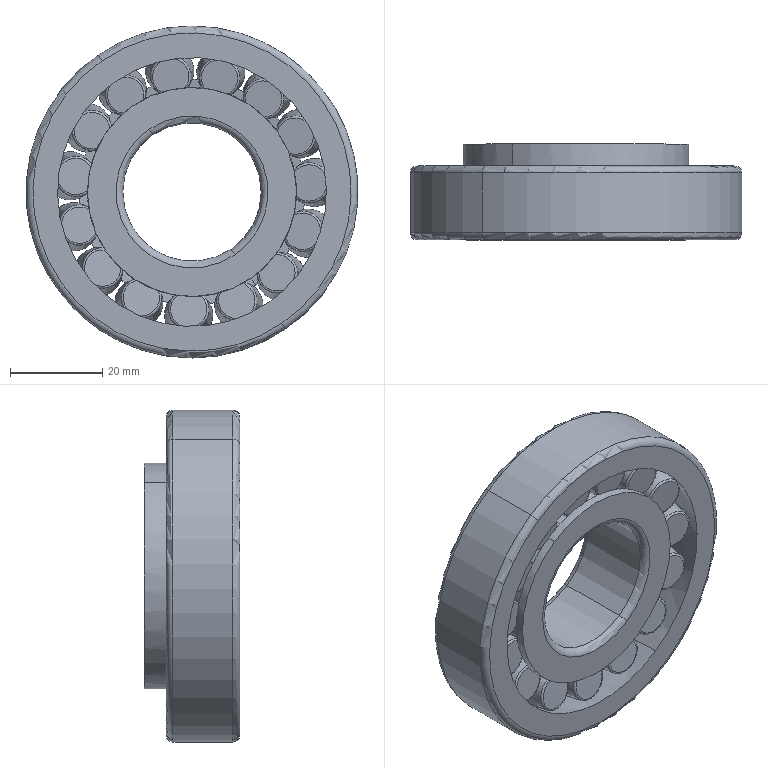Part | NX | features BREP 1 | 1 solid | 148 faces | box 72 x 20.75 x 72 mm | volume 45638 mm3 | torus 68 | cone 38 | plane 34 | cylinder 8 | commonest cylinder face diameters 30 x2 45.307 x2 49.001 x2 72 x2